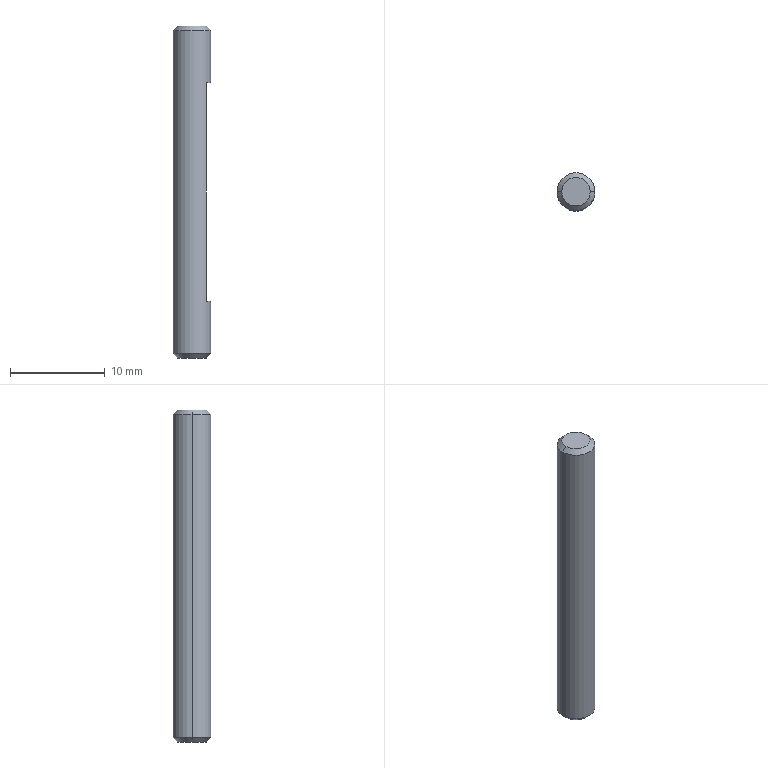Part | SolidWorks | features Chamfer 1, Extrusion 1, ICE 1 | 1 solid | 11 faces | box 4 x 4 x 35 mm | volume 416.091 mm3 | plane 5 | cone 4 | cylinder 2 | commonest cylinder face diameters 4 x2
STEP:
#1=CARTESIAN_POINT('',(1.5,0.,17.5));
#2=VERTEX_POINT('',#1);
#3=CARTESIAN_POINT('',(-1.5,0.,17.5));
#4=VERTEX_POINT('',#3);
#5=CARTESIAN_POINT('',(0.,0.,17.5));
#6=DIRECTION('',(0.,0.,1.));
#7=DIRECTION('',(1.,0.,0.));
#8=AXIS2_PLACEMENT_3D('',#5,#6,#7);
#9=CIRCLE('',#8,1.5);
#10=EDGE_CURVE('',#2,#4,#9,.T.);
#11=ORIENTED_EDGE('',*,*,#10,.F.);
#12=CARTESIAN_POINT('',(2.,0.,17.));
#13=VERTEX_POINT('',#12);
#14=CARTESIAN_POINT('',(1.5,0.,17.5));
#15=DIRECTION('',(0.7071,0.,-0.7071));
#16=VECTOR('',#15,1000.);
#17=LINE('',#14,#16);
#18=EDGE_CURVE('',#2,#13,#17,.T.);
#19=ORIENTED_EDGE('',*,*,#18,.T.);
#20=CARTESIAN_POINT('',(-2.,0.,17.));
#21=VERTEX_POINT('',#20);
#22=CARTESIAN_POINT('',(0.,0.,17.));
#23=DIRECTION('',(0.,0.,-1.));
#24=DIRECTION('',(1.,0.,0.));
#25=AXIS2_PLACEMENT_3D('',#22,#23,#24);
#26=CIRCLE('',#25,2.);
#27=EDGE_CURVE('',#21,#13,#26,.T.);
#28=ORIENTED_EDGE('',*,*,#27,.F.);
#29=CARTESIAN_POINT('',(-1.5,0.,17.5));
#30=DIRECTION('',(-0.7071,0.,-0.7071));
#31=VECTOR('',#30,1000.);
#32=LINE('',#29,#31);
#33=EDGE_CURVE('',#4,#21,#32,.T.);
#34=ORIENTED_EDGE('',*,*,#33,.F.);
#35=EDGE_LOOP('',(#11,#19,#28,#34));
#36=FACE_OUTER_BOUND('',#35,.T.);
#37=CARTESIAN_POINT('',(0.,0.,17.5));
#38=DIRECTION('',(0.,0.,-1.));
#39=DIRECTION('',(-1.,0.,0.));
#40=AXIS2_PLACEMENT_3D('',#37,#38,#39);
#41=CONICAL_SURFACE('',#40,1.5,0.7854);
#42=ADVANCED_FACE('',(#36),#41,.T.);
#43=CARTESIAN_POINT('',(-1.5,0.,-17.5));
#44=VERTEX_POINT('',#43);
#45=CARTESIAN_POINT('',(1.5,0.,-17.5));
#46=VERTEX_POINT('',#45);
#47=CARTESIAN_POINT('',(0.,0.,-17.5));
#48=DIRECTION('',(0.,0.,-1.));
#49=DIRECTION('',(1.,0.,0.));
#50=AXIS2_PLACEMENT_3D('',#47,#48,#49);
#51=CIRCLE('',#50,1.5);
#52=EDGE_CURVE('',#44,#46,#51,.T.);
#53=ORIENTED_EDGE('',*,*,#52,.F.);
#54=CARTESIAN_POINT('',(-2.,0.,-17.));
#55=VERTEX_POINT('',#54);
#56=CARTESIAN_POINT('',(-2.,0.,-17.));
#57=DIRECTION('',(-0.7071,0.,0.7071));
#58=VECTOR('',#57,1000.);
#59=LINE('',#56,#58);
#60=EDGE_CURVE('',#44,#55,#59,.T.);
#61=ORIENTED_EDGE('',*,*,#60,.T.);
#62=CARTESIAN_POINT('',(2.,0.,-17.));
#63=VERTEX_POINT('',#62);
#64=CARTESIAN_POINT('',(0.,0.,-17.));
#65=DIRECTION('',(0.,0.,1.));
#66=DIRECTION('',(1.,0.,0.));
#67=AXIS2_PLACEMENT_3D('',#64,#65,#66);
#68=CIRCLE('',#67,2.);
#69=EDGE_CURVE('',#63,#55,#68,.T.);
#70=ORIENTED_EDGE('',*,*,#69,.F.);
#71=CARTESIAN_POINT('',(2.,0.,-17.));
#72=DIRECTION('',(0.7071,0.,0.7071));
#73=VECTOR('',#72,1000.);
#74=LINE('',#71,#73);
#75=EDGE_CURVE('',#46,#63,#74,.T.);
#76=ORIENTED_EDGE('',*,*,#75,.F.);
#77=EDGE_LOOP('',(#53,#61,#70,#76));
#78=FACE_OUTER_BOUND('',#77,.T.);
#79=CARTESIAN_POINT('',(0.,0.,-17.));
#80=DIRECTION('',(0.,0.,1.));
#81=DIRECTION('',(1.,0.,0.));
#82=AXIS2_PLACEMENT_3D('',#79,#80,#81);
#83=CONICAL_SURFACE('',#82,2.,0.7854);
#84=ADVANCED_FACE('',(#78),#83,.T.);
#85=ORIENTED_EDGE('',*,*,#27,.T.);
#86=CARTESIAN_POINT('',(2.,0.,11.5));
#87=VERTEX_POINT('',#86);
#88=CARTESIAN_POINT('',(2.,0.,17.5));
#89=DIRECTION('',(0.,0.,-1.));
#90=VECTOR('',#89,1000.);
#91=LINE('',#88,#90);
#92=EDGE_CURVE('',#13,#87,#91,.T.);
#93=ORIENTED_EDGE('',*,*,#92,.T.);
#94=CARTESIAN_POINT('',(1.5,1.323,11.5));
#95=VERTEX_POINT('',#94);
#96=CARTESIAN_POINT('',(0.,0.,11.5));
#97=DIRECTION('',(0.,0.,1.));
#98=DIRECTION('',(1.,0.,0.));
#99=AXIS2_PLACEMENT_3D('',#96,#97,#98);
#100=CIRCLE('',#99,2.);
#101=EDGE_CURVE('',#87,#95,#100,.T.);
#102=ORIENTED_EDGE('',*,*,#101,.T.);
#103=CARTESIAN_POINT('',(1.5,1.323,-11.5));
#104=VERTEX_POINT('',#103);
#105=CARTESIAN_POINT('',(1.5,1.323,17.5));
#106=DIRECTION('',(0.,0.,-1.));
#107=VECTOR('',#106,1000.);
#108=LINE('',#105,#107);
#109=EDGE_CURVE('',#95,#104,#108,.T.);
#110=ORIENTED_EDGE('',*,*,#109,.T.);
#111=CARTESIAN_POINT('',(2.,0.,-11.5));
#112=VERTEX_POINT('',#111);
#113=CARTESIAN_POINT('',(0.,0.,-11.5));
#114=DIRECTION('',(0.,0.,-1.));
#115=DIRECTION('',(-1.,0.,0.));
#116=AXIS2_PLACEMENT_3D('',#113,#114,#115);
#117=CIRCLE('',#116,2.);
#118=EDGE_CURVE('',#104,#112,#117,.T.);
#119=ORIENTED_EDGE('',*,*,#118,.T.);
#120=CARTESIAN_POINT('',(2.,0.,17.5));
#121=DIRECTION('',(0.,0.,-1.));
#122=VECTOR('',#121,1000.);
#123=LINE('',#120,#122);
#124=EDGE_CURVE('',#112,#63,#123,.T.);
#125=ORIENTED_EDGE('',*,*,#124,.T.);
#126=ORIENTED_EDGE('',*,*,#69,.T.);
#127=CARTESIAN_POINT('',(-2.,0.,17.5));
#128=DIRECTION('',(0.,0.,-1.));
#129=VECTOR('',#128,1000.);
#130=LINE('',#127,#129);
#131=EDGE_CURVE('',#21,#55,#130,.T.);
#132=ORIENTED_EDGE('',*,*,#131,.F.);
#133=EDGE_LOOP('',(#85,#93,#102,#110,#119,#125,#126,#132));
#134=FACE_OUTER_BOUND('',#133,.T.);
#135=CARTESIAN_POINT('',(0.,0.,17.5));
#136=DIRECTION('',(0.,0.,-1.));
#137=DIRECTION('',(-1.,0.,0.));
#138=AXIS2_PLACEMENT_3D('',#135,#136,#137);
#139=CYLINDRICAL_SURFACE('',#138,2.);
#140=ADVANCED_FACE('',(#134),#139,.T.);
#141=ORIENTED_EDGE('',*,*,#92,.F.);
#142=CARTESIAN_POINT('',(0.,0.,17.));
#143=DIRECTION('',(0.,0.,-1.));
#144=DIRECTION('',(1.,0.,0.));
#145=AXIS2_PLACEMENT_3D('',#142,#143,#144);
#146=CIRCLE('',#145,2.);
#147=EDGE_CURVE('',#13,#21,#146,.T.);
#148=ORIENTED_EDGE('',*,*,#147,.T.);
#149=ORIENTED_EDGE('',*,*,#131,.T.);
#150=CARTESIAN_POINT('',(0.,0.,-17.));
#151=DIRECTION('',(0.,0.,1.));
#152=DIRECTION('',(1.,0.,0.));
#153=AXIS2_PLACEMENT_3D('',#150,#151,#152);
#154=CIRCLE('',#153,2.);
#155=EDGE_CURVE('',#55,#63,#154,.T.);
#156=ORIENTED_EDGE('',*,*,#155,.T.);
#157=ORIENTED_EDGE('',*,*,#124,.F.);
#158=CARTESIAN_POINT('',(1.5,-1.323,-11.5));
#159=VERTEX_POINT('',#158);
#160=CARTESIAN_POINT('',(0.,0.,-11.5));
#161=DIRECTION('',(0.,0.,-1.));
#162=DIRECTION('',(-1.,0.,0.));
#163=AXIS2_PLACEMENT_3D('',#160,#161,#162);
#164=CIRCLE('',#163,2.);
#165=EDGE_CURVE('',#112,#159,#164,.T.);
#166=ORIENTED_EDGE('',*,*,#165,.T.);
#167=CARTESIAN_POINT('',(1.5,-1.323,11.5));
#168=VERTEX_POINT('',#167);
#169=CARTESIAN_POINT('',(1.5,-1.323,17.5));
#170=DIRECTION('',(0.,0.,1.));
#171=VECTOR('',#170,1000.);
#172=LINE('',#169,#171);
#173=EDGE_CURVE('',#159,#168,#172,.T.);
#174=ORIENTED_EDGE('',*,*,#173,.T.);
#175=CARTESIAN_POINT('',(0.,0.,11.5));
#176=DIRECTION('',(0.,0.,1.));
#177=DIRECTION('',(1.,0.,0.));
#178=AXIS2_PLACEMENT_3D('',#175,#176,#177);
#179=CIRCLE('',#178,2.);
#180=EDGE_CURVE('',#168,#87,#179,.T.);
#181=ORIENTED_EDGE('',*,*,#180,.T.);
#182=EDGE_LOOP('',(#141,#148,#149,#156,#157,#166,#174,#181));
#183=FACE_OUTER_BOUND('',#182,.T.);
#184=CARTESIAN_POINT('',(0.,0.,17.5));
#185=DIRECTION('',(0.,0.,-1.));
#186=DIRECTION('',(-1.,0.,0.));
#187=AXIS2_PLACEMENT_3D('',#184,#185,#186);
#188=CYLINDRICAL_SURFACE('',#187,2.);
#189=ADVANCED_FACE('',(#183),#188,.T.);
#190=CARTESIAN_POINT('',(0.,0.,17.5));
#191=DIRECTION('',(0.,0.,1.));
#192=DIRECTION('',(1.,0.,0.));
#193=AXIS2_PLACEMENT_3D('',#190,#191,#192);
#194=CIRCLE('',#193,1.5);
#195=EDGE_CURVE('',#4,#2,#194,.T.);
#196=ORIENTED_EDGE('',*,*,#195,.T.);
#197=ORIENTED_EDGE('',*,*,#10,.T.);
#198=EDGE_LOOP('',(#196,#197));
#199=FACE_OUTER_BOUND('',#198,.T.);
#200=CARTESIAN_POINT('',(0.,0.,17.5));
#201=DIRECTION('',(0.,0.,1.));
#202=DIRECTION('',(1.,0.,0.));
#203=AXIS2_PLACEMENT_3D('',#200,#201,#202);
#204=PLANE('',#203);
#205=ADVANCED_FACE('',(#199),#204,.T.);
#206=CARTESIAN_POINT('',(0.,0.,-17.5));
#207=DIRECTION('',(0.,0.,-1.));
#208=DIRECTION('',(1.,0.,0.));
#209=AXIS2_PLACEMENT_3D('',#206,#207,#208);
#210=CIRCLE('',#209,1.5);
#211=EDGE_CURVE('',#46,#44,#210,.T.);
#212=ORIENTED_EDGE('',*,*,#211,.T.);
#213=ORIENTED_EDGE('',*,*,#52,.T.);
#214=EDGE_LOOP('',(#212,#213));
#215=FACE_OUTER_BOUND('',#214,.T.);
#216=CARTESIAN_POINT('',(0.,0.,-17.5));
#217=DIRECTION('',(0.,0.,1.));
#218=DIRECTION('',(1.,0.,0.));
#219=AXIS2_PLACEMENT_3D('',#216,#217,#218);
#220=PLANE('',#219);
#221=ADVANCED_FACE('',(#215),#220,.F.);
#222=ORIENTED_EDGE('',*,*,#60,.F.);
#223=ORIENTED_EDGE('',*,*,#211,.F.);
#224=ORIENTED_EDGE('',*,*,#75,.T.);
#225=ORIENTED_EDGE('',*,*,#155,.F.);
#226=EDGE_LOOP('',(#222,#223,#224,#225));
#227=FACE_OUTER_BOUND('',#226,.T.);
#228=CARTESIAN_POINT('',(0.,0.,-17.));
#229=DIRECTION('',(0.,0.,1.));
#230=DIRECTION('',(1.,0.,0.));
#231=AXIS2_PLACEMENT_3D('',#228,#229,#230);
#232=CONICAL_SURFACE('',#231,2.,0.7854);
#233=ADVANCED_FACE('',(#227),#232,.T.);
#234=ORIENTED_EDGE('',*,*,#18,.F.);
#235=ORIENTED_EDGE('',*,*,#195,.F.);
#236=ORIENTED_EDGE('',*,*,#33,.T.);
#237=ORIENTED_EDGE('',*,*,#147,.F.);
#238=EDGE_LOOP('',(#234,#235,#236,#237));
#239=FACE_OUTER_BOUND('',#238,.T.);
#240=CARTESIAN_POINT('',(0.,0.,17.5));
#241=DIRECTION('',(0.,0.,-1.));
#242=DIRECTION('',(-1.,0.,0.));
#243=AXIS2_PLACEMENT_3D('',#240,#241,#242);
#244=CONICAL_SURFACE('',#243,1.5,0.7854);
#245=ADVANCED_FACE('',(#239),#244,.T.);
#246=CARTESIAN_POINT('',(1.5,-5.,11.5));
#247=DIRECTION('',(0.,1.,0.));
#248=VECTOR('',#247,1000.);
#249=LINE('',#246,#248);
#250=EDGE_CURVE('',#168,#95,#249,.T.);
#251=ORIENTED_EDGE('',*,*,#250,.F.);
#252=ORIENTED_EDGE('',*,*,#173,.F.);
#253=CARTESIAN_POINT('',(1.5,-5.,-11.5));
#254=DIRECTION('',(0.,1.,0.));
#255=VECTOR('',#254,1000.);
#256=LINE('',#253,#255);
#257=EDGE_CURVE('',#159,#104,#256,.T.);
#258=ORIENTED_EDGE('',*,*,#257,.T.);
#259=ORIENTED_EDGE('',*,*,#109,.F.);
#260=EDGE_LOOP('',(#251,#252,#258,#259));
#261=FACE_OUTER_BOUND('',#260,.T.);
#262=CARTESIAN_POINT('',(1.5,-5.,11.5));
#263=DIRECTION('',(-1.,0.,0.));
#264=DIRECTION('',(0.,0.,1.));
#265=AXIS2_PLACEMENT_3D('',#262,#263,#264);
#266=PLANE('',#265);
#267=ADVANCED_FACE('',(#261),#266,.F.);
#268=ORIENTED_EDGE('',*,*,#257,.F.);
#269=ORIENTED_EDGE('',*,*,#165,.F.);
#270=ORIENTED_EDGE('',*,*,#118,.F.);
#271=EDGE_LOOP('',(#268,#269,#270));
#272=FACE_OUTER_BOUND('',#271,.T.);
#273=CARTESIAN_POINT('',(2.5,-5.,-11.5));
#274=DIRECTION('',(0.,0.,-1.));
#275=DIRECTION('',(-1.,0.,0.));
#276=AXIS2_PLACEMENT_3D('',#273,#274,#275);
#277=PLANE('',#276);
#278=ADVANCED_FACE('',(#272),#277,.F.);
#279=ORIENTED_EDGE('',*,*,#250,.T.);
#280=ORIENTED_EDGE('',*,*,#101,.F.);
#281=ORIENTED_EDGE('',*,*,#180,.F.);
#282=EDGE_LOOP('',(#279,#280,#281));
#283=FACE_OUTER_BOUND('',#282,.T.);
#284=CARTESIAN_POINT('',(2.5,-5.,11.5));
#285=DIRECTION('',(0.,0.,1.));
#286=DIRECTION('',(1.,0.,0.));
#287=AXIS2_PLACEMENT_3D('',#284,#285,#286);
#288=PLANE('',#287);
#289=ADVANCED_FACE('',(#283),#288,.F.);
#290=CLOSED_SHELL('',(#42,#84,#140,#189,#205,#221,#233,#245,#267,#278,#289));
#291=MANIFOLD_SOLID_BREP('',#290);
#292=CARTESIAN_POINT('',(0.,0.,0.));
#293=DIRECTION('',(0.,0.,1.));
#294=DIRECTION('',(1.,0.,0.));
#295=AXIS2_PLACEMENT_3D('',#292,#293,#294);
#296=(LENGTH_UNIT()NAMED_UNIT(*)SI_UNIT(.MILLI.,.METRE.));
#297=UNCERTAINTY_MEASURE_WITH_UNIT(LENGTH_MEASURE(0.00001),#296,'','');
#298=(NAMED_UNIT(*)PLANE_ANGLE_UNIT()SI_UNIT($,.RADIAN.));
#299=(NAMED_UNIT(*)SI_UNIT($,.STERADIAN.)SOLID_ANGLE_UNIT());
#300=(GEOMETRIC_REPRESENTATION_CONTEXT(3)GLOBAL_UNCERTAINTY_ASSIGNED_CONTEXT((#297))GLOBAL_UNIT_ASSIGNED_CONTEXT((#296,#298,#299))REPRESENTATION_CONTEXT('',''));
#301=ADVANCED_BREP_SHAPE_REPRESENTATION('',(#291,#295),#300);